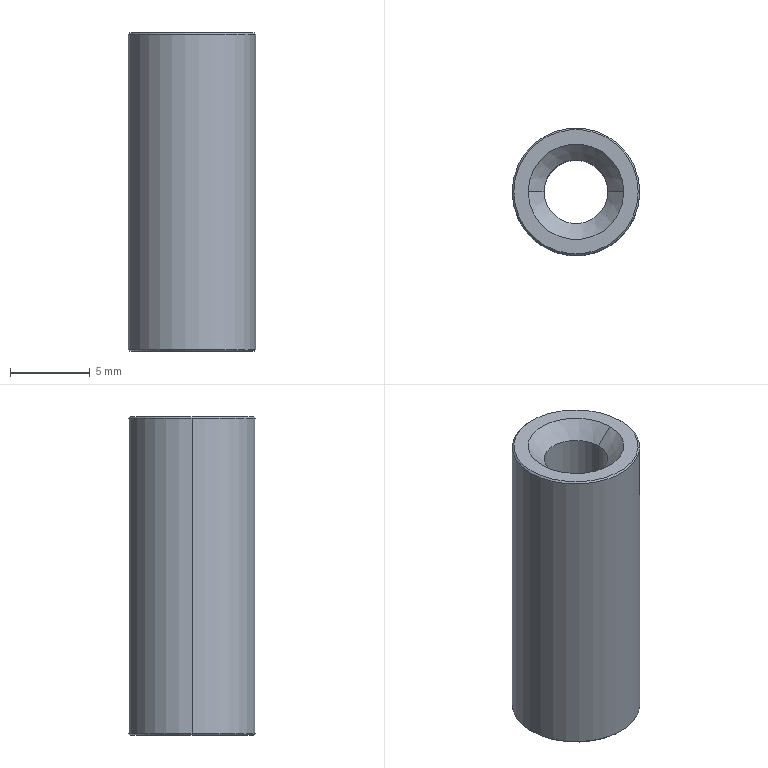Part | NX | features BREP 1 | 1 solid | 14 faces | box 8 x 8 x 20 mm | volume 739.072 mm3 | cone 8 | cylinder 4 | plane 2 | commonest cylinder face diameters 4 x2 8 x2
STEP:
#1=CARTESIAN_POINT('',(2.,0.,1.));
#2=VERTEX_POINT('',#1);
#3=CARTESIAN_POINT('',(-2.,0.,1.));
#4=VERTEX_POINT('',#3);
#5=CARTESIAN_POINT('',(0.,0.,1.));
#6=DIRECTION('',(0.,0.,-1.));
#7=DIRECTION('',(1.,0.,0.));
#8=AXIS2_PLACEMENT_3D('',#5,#6,#7);
#9=CIRCLE('',#8,2.);
#10=EDGE_CURVE('',#2,#4,#9,.T.);
#11=ORIENTED_EDGE('',*,*,#10,.F.);
#12=CARTESIAN_POINT('',(3.,0.,0.));
#13=VERTEX_POINT('',#12);
#14=CARTESIAN_POINT('',(3.,0.,0.));
#15=DIRECTION('',(0.7071,0.,-0.7071));
#16=VECTOR('',#15,1000.);
#17=LINE('',#14,#16);
#18=EDGE_CURVE('',#2,#13,#17,.T.);
#19=ORIENTED_EDGE('',*,*,#18,.T.);
#20=CARTESIAN_POINT('',(-3.,0.,0.));
#21=VERTEX_POINT('',#20);
#22=CARTESIAN_POINT('',(0.,0.,0.));
#23=DIRECTION('',(0.,0.,1.));
#24=DIRECTION('',(1.,0.,0.));
#25=AXIS2_PLACEMENT_3D('',#22,#23,#24);
#26=CIRCLE('',#25,3.);
#27=EDGE_CURVE('',#21,#13,#26,.T.);
#28=ORIENTED_EDGE('',*,*,#27,.F.);
#29=CARTESIAN_POINT('',(-3.,0.,0.));
#30=DIRECTION('',(-0.7071,0.,-0.7071));
#31=VECTOR('',#30,1000.);
#32=LINE('',#29,#31);
#33=EDGE_CURVE('',#4,#21,#32,.T.);
#34=ORIENTED_EDGE('',*,*,#33,.F.);
#35=EDGE_LOOP('',(#11,#19,#28,#34));
#36=FACE_BOUND('',#35,.T.);
#37=CARTESIAN_POINT('',(0.,0.,0.));
#38=DIRECTION('',(0.,0.,-1.));
#39=DIRECTION('',(-1.,0.,0.));
#40=AXIS2_PLACEMENT_3D('',#37,#38,#39);
#41=CONICAL_SURFACE('',#40,3.,0.7854);
#42=ADVANCED_FACE('',(#36),#41,.F.);
#43=CARTESIAN_POINT('',(-2.,0.,19.));
#44=VERTEX_POINT('',#43);
#45=CARTESIAN_POINT('',(2.,0.,19.));
#46=VERTEX_POINT('',#45);
#47=CARTESIAN_POINT('',(0.,0.,19.));
#48=DIRECTION('',(0.,0.,1.));
#49=DIRECTION('',(1.,0.,0.));
#50=AXIS2_PLACEMENT_3D('',#47,#48,#49);
#51=CIRCLE('',#50,2.);
#52=EDGE_CURVE('',#44,#46,#51,.T.);
#53=ORIENTED_EDGE('',*,*,#52,.F.);
#54=CARTESIAN_POINT('',(-3.,0.,20.));
#55=VERTEX_POINT('',#54);
#56=CARTESIAN_POINT('',(-2.,0.,19.));
#57=DIRECTION('',(-0.7071,0.,0.7071));
#58=VECTOR('',#57,1000.);
#59=LINE('',#56,#58);
#60=EDGE_CURVE('',#55,#44,#59,.F.);
#61=ORIENTED_EDGE('',*,*,#60,.F.);
#62=CARTESIAN_POINT('',(3.,0.,20.));
#63=VERTEX_POINT('',#62);
#64=CARTESIAN_POINT('',(0.,0.,20.));
#65=DIRECTION('',(0.,0.,-1.));
#66=DIRECTION('',(1.,0.,0.));
#67=AXIS2_PLACEMENT_3D('',#64,#65,#66);
#68=CIRCLE('',#67,3.);
#69=EDGE_CURVE('',#63,#55,#68,.T.);
#70=ORIENTED_EDGE('',*,*,#69,.F.);
#71=CARTESIAN_POINT('',(2.,0.,19.));
#72=DIRECTION('',(0.7071,0.,0.7071));
#73=VECTOR('',#72,1000.);
#74=LINE('',#71,#73);
#75=EDGE_CURVE('',#63,#46,#74,.F.);
#76=ORIENTED_EDGE('',*,*,#75,.T.);
#77=EDGE_LOOP('',(#53,#61,#70,#76));
#78=FACE_BOUND('',#77,.T.);
#79=CARTESIAN_POINT('',(0.,0.,19.));
#80=DIRECTION('',(0.,0.,1.));
#81=DIRECTION('',(1.,0.,0.));
#82=AXIS2_PLACEMENT_3D('',#79,#80,#81);
#83=CONICAL_SURFACE('',#82,2.,0.7854);
#84=ADVANCED_FACE('',(#78),#83,.F.);
#85=CARTESIAN_POINT('',(3.9,0.,20.));
#86=VERTEX_POINT('',#85);
#87=CARTESIAN_POINT('',(-3.9,0.,20.));
#88=VERTEX_POINT('',#87);
#89=CARTESIAN_POINT('',(0.,0.,20.));
#90=DIRECTION('',(0.,0.,1.));
#91=DIRECTION('',(1.,0.,0.));
#92=AXIS2_PLACEMENT_3D('',#89,#90,#91);
#93=CIRCLE('',#92,3.9);
#94=EDGE_CURVE('',#86,#88,#93,.T.);
#95=ORIENTED_EDGE('',*,*,#94,.F.);
#96=CARTESIAN_POINT('',(4.,0.,19.9));
#97=VERTEX_POINT('',#96);
#98=CARTESIAN_POINT('',(3.9,0.,20.));
#99=DIRECTION('',(0.7071,0.,-0.7071));
#100=VECTOR('',#99,1000.);
#101=LINE('',#98,#100);
#102=EDGE_CURVE('',#86,#97,#101,.T.);
#103=ORIENTED_EDGE('',*,*,#102,.T.);
#104=CARTESIAN_POINT('',(-4.,0.,19.9));
#105=VERTEX_POINT('',#104);
#106=CARTESIAN_POINT('',(0.,0.,19.9));
#107=DIRECTION('',(0.,0.,-1.));
#108=DIRECTION('',(1.,0.,0.));
#109=AXIS2_PLACEMENT_3D('',#106,#107,#108);
#110=CIRCLE('',#109,4.);
#111=EDGE_CURVE('',#105,#97,#110,.T.);
#112=ORIENTED_EDGE('',*,*,#111,.F.);
#113=CARTESIAN_POINT('',(-3.9,0.,20.));
#114=DIRECTION('',(-0.7071,0.,-0.7071));
#115=VECTOR('',#114,1000.);
#116=LINE('',#113,#115);
#117=EDGE_CURVE('',#88,#105,#116,.T.);
#118=ORIENTED_EDGE('',*,*,#117,.F.);
#119=EDGE_LOOP('',(#95,#103,#112,#118));
#120=FACE_BOUND('',#119,.T.);
#121=CARTESIAN_POINT('',(0.,0.,20.));
#122=DIRECTION('',(0.,0.,-1.));
#123=DIRECTION('',(-1.,0.,0.));
#124=AXIS2_PLACEMENT_3D('',#121,#122,#123);
#125=CONICAL_SURFACE('',#124,3.9,0.7854);
#126=ADVANCED_FACE('',(#120),#125,.T.);
#127=CARTESIAN_POINT('',(-3.9,0.,0.));
#128=VERTEX_POINT('',#127);
#129=CARTESIAN_POINT('',(3.9,0.,0.));
#130=VERTEX_POINT('',#129);
#131=CARTESIAN_POINT('',(0.,0.,0.));
#132=DIRECTION('',(0.,0.,-1.));
#133=DIRECTION('',(1.,0.,0.));
#134=AXIS2_PLACEMENT_3D('',#131,#132,#133);
#135=CIRCLE('',#134,3.9);
#136=EDGE_CURVE('',#128,#130,#135,.T.);
#137=ORIENTED_EDGE('',*,*,#136,.F.);
#138=CARTESIAN_POINT('',(-4.,0.,0.1));
#139=VERTEX_POINT('',#138);
#140=CARTESIAN_POINT('',(-4.,0.,0.1));
#141=DIRECTION('',(-0.7071,0.,0.7071));
#142=VECTOR('',#141,1000.);
#143=LINE('',#140,#142);
#144=EDGE_CURVE('',#139,#128,#143,.F.);
#145=ORIENTED_EDGE('',*,*,#144,.F.);
#146=CARTESIAN_POINT('',(4.,0.,0.1));
#147=VERTEX_POINT('',#146);
#148=CARTESIAN_POINT('',(0.,0.,0.1));
#149=DIRECTION('',(0.,0.,1.));
#150=DIRECTION('',(1.,0.,0.));
#151=AXIS2_PLACEMENT_3D('',#148,#149,#150);
#152=CIRCLE('',#151,4.);
#153=EDGE_CURVE('',#147,#139,#152,.T.);
#154=ORIENTED_EDGE('',*,*,#153,.F.);
#155=CARTESIAN_POINT('',(4.,0.,0.1));
#156=DIRECTION('',(0.7071,0.,0.7071));
#157=VECTOR('',#156,1000.);
#158=LINE('',#155,#157);
#159=EDGE_CURVE('',#147,#130,#158,.F.);
#160=ORIENTED_EDGE('',*,*,#159,.T.);
#161=EDGE_LOOP('',(#137,#145,#154,#160));
#162=FACE_BOUND('',#161,.T.);
#163=CARTESIAN_POINT('',(0.,0.,0.1));
#164=DIRECTION('',(0.,0.,1.));
#165=DIRECTION('',(1.,0.,0.));
#166=AXIS2_PLACEMENT_3D('',#163,#164,#165);
#167=CONICAL_SURFACE('',#166,4.,0.7854);
#168=ADVANCED_FACE('',(#162),#167,.T.);
#169=ORIENTED_EDGE('',*,*,#52,.T.);
#170=CARTESIAN_POINT('',(2.,0.,20.));
#171=DIRECTION('',(0.,0.,-1.));
#172=VECTOR('',#171,1000.);
#173=LINE('',#170,#172);
#174=EDGE_CURVE('',#46,#2,#173,.T.);
#175=ORIENTED_EDGE('',*,*,#174,.T.);
#176=ORIENTED_EDGE('',*,*,#10,.T.);
#177=CARTESIAN_POINT('',(-2.,0.,20.));
#178=DIRECTION('',(0.,0.,-1.));
#179=VECTOR('',#178,1000.);
#180=LINE('',#177,#179);
#181=EDGE_CURVE('',#44,#4,#180,.T.);
#182=ORIENTED_EDGE('',*,*,#181,.F.);
#183=EDGE_LOOP('',(#169,#175,#176,#182));
#184=FACE_BOUND('',#183,.T.);
#185=CARTESIAN_POINT('',(0.,0.,20.));
#186=DIRECTION('',(0.,0.,-1.));
#187=DIRECTION('',(-1.,0.,0.));
#188=AXIS2_PLACEMENT_3D('',#185,#186,#187);
#189=CYLINDRICAL_SURFACE('',#188,2.);
#190=ADVANCED_FACE('',(#184),#189,.F.);
#191=ORIENTED_EDGE('',*,*,#111,.T.);
#192=CARTESIAN_POINT('',(4.,0.,20.));
#193=DIRECTION('',(0.,0.,-1.));
#194=VECTOR('',#193,1000.);
#195=LINE('',#192,#194);
#196=EDGE_CURVE('',#97,#147,#195,.T.);
#197=ORIENTED_EDGE('',*,*,#196,.T.);
#198=ORIENTED_EDGE('',*,*,#153,.T.);
#199=CARTESIAN_POINT('',(-4.,0.,20.));
#200=DIRECTION('',(0.,0.,-1.));
#201=VECTOR('',#200,1000.);
#202=LINE('',#199,#201);
#203=EDGE_CURVE('',#105,#139,#202,.T.);
#204=ORIENTED_EDGE('',*,*,#203,.F.);
#205=EDGE_LOOP('',(#191,#197,#198,#204));
#206=FACE_BOUND('',#205,.T.);
#207=CARTESIAN_POINT('',(0.,0.,20.));
#208=DIRECTION('',(0.,0.,-1.));
#209=DIRECTION('',(-1.,0.,0.));
#210=AXIS2_PLACEMENT_3D('',#207,#208,#209);
#211=CYLINDRICAL_SURFACE('',#210,4.);
#212=ADVANCED_FACE('',(#206),#211,.T.);
#213=CARTESIAN_POINT('',(0.,0.,20.));
#214=DIRECTION('',(0.,0.,1.));
#215=DIRECTION('',(1.,0.,0.));
#216=AXIS2_PLACEMENT_3D('',#213,#214,#215);
#217=CIRCLE('',#216,3.9);
#218=EDGE_CURVE('',#88,#86,#217,.T.);
#219=ORIENTED_EDGE('',*,*,#218,.T.);
#220=ORIENTED_EDGE('',*,*,#94,.T.);
#221=EDGE_LOOP('',(#219,#220));
#222=FACE_BOUND('',#221,.T.);
#223=ORIENTED_EDGE('',*,*,#69,.T.);
#224=CARTESIAN_POINT('',(0.,0.,20.));
#225=DIRECTION('',(0.,0.,-1.));
#226=DIRECTION('',(1.,0.,0.));
#227=AXIS2_PLACEMENT_3D('',#224,#225,#226);
#228=CIRCLE('',#227,3.);
#229=EDGE_CURVE('',#55,#63,#228,.T.);
#230=ORIENTED_EDGE('',*,*,#229,.T.);
#231=EDGE_LOOP('',(#223,#230));
#232=FACE_BOUND('',#231,.T.);
#233=CARTESIAN_POINT('',(0.,0.,20.));
#234=DIRECTION('',(0.,0.,1.));
#235=DIRECTION('',(1.,0.,0.));
#236=AXIS2_PLACEMENT_3D('',#233,#234,#235);
#237=PLANE('',#236);
#238=ADVANCED_FACE('',(#222,#232),#237,.T.);
#239=CARTESIAN_POINT('',(0.,0.,0.));
#240=DIRECTION('',(0.,0.,-1.));
#241=DIRECTION('',(1.,0.,0.));
#242=AXIS2_PLACEMENT_3D('',#239,#240,#241);
#243=CIRCLE('',#242,3.9);
#244=EDGE_CURVE('',#130,#128,#243,.T.);
#245=ORIENTED_EDGE('',*,*,#244,.T.);
#246=ORIENTED_EDGE('',*,*,#136,.T.);
#247=EDGE_LOOP('',(#245,#246));
#248=FACE_BOUND('',#247,.T.);
#249=ORIENTED_EDGE('',*,*,#27,.T.);
#250=CARTESIAN_POINT('',(0.,0.,0.));
#251=DIRECTION('',(0.,0.,1.));
#252=DIRECTION('',(1.,0.,0.));
#253=AXIS2_PLACEMENT_3D('',#250,#251,#252);
#254=CIRCLE('',#253,3.);
#255=EDGE_CURVE('',#13,#21,#254,.T.);
#256=ORIENTED_EDGE('',*,*,#255,.T.);
#257=EDGE_LOOP('',(#249,#256));
#258=FACE_BOUND('',#257,.T.);
#259=CARTESIAN_POINT('',(0.,0.,0.));
#260=DIRECTION('',(0.,0.,1.));
#261=DIRECTION('',(1.,0.,0.));
#262=AXIS2_PLACEMENT_3D('',#259,#260,#261);
#263=PLANE('',#262);
#264=ADVANCED_FACE('',(#248,#258),#263,.F.);
#265=ORIENTED_EDGE('',*,*,#196,.F.);
#266=CARTESIAN_POINT('',(0.,0.,19.9));
#267=DIRECTION('',(0.,0.,-1.));
#268=DIRECTION('',(1.,0.,0.));
#269=AXIS2_PLACEMENT_3D('',#266,#267,#268);
#270=CIRCLE('',#269,4.);
#271=EDGE_CURVE('',#97,#105,#270,.T.);
#272=ORIENTED_EDGE('',*,*,#271,.T.);
#273=ORIENTED_EDGE('',*,*,#203,.T.);
#274=CARTESIAN_POINT('',(0.,0.,0.1));
#275=DIRECTION('',(0.,0.,1.));
#276=DIRECTION('',(1.,0.,0.));
#277=AXIS2_PLACEMENT_3D('',#274,#275,#276);
#278=CIRCLE('',#277,4.);
#279=EDGE_CURVE('',#139,#147,#278,.T.);
#280=ORIENTED_EDGE('',*,*,#279,.T.);
#281=EDGE_LOOP('',(#265,#272,#273,#280));
#282=FACE_BOUND('',#281,.T.);
#283=CARTESIAN_POINT('',(0.,0.,20.));
#284=DIRECTION('',(0.,0.,-1.));
#285=DIRECTION('',(-1.,0.,0.));
#286=AXIS2_PLACEMENT_3D('',#283,#284,#285);
#287=CYLINDRICAL_SURFACE('',#286,4.);
#288=ADVANCED_FACE('',(#282),#287,.T.);
#289=ORIENTED_EDGE('',*,*,#174,.F.);
#290=CARTESIAN_POINT('',(0.,0.,19.));
#291=DIRECTION('',(0.,0.,1.));
#292=DIRECTION('',(1.,0.,0.));
#293=AXIS2_PLACEMENT_3D('',#290,#291,#292);
#294=CIRCLE('',#293,2.);
#295=EDGE_CURVE('',#46,#44,#294,.T.);
#296=ORIENTED_EDGE('',*,*,#295,.T.);
#297=ORIENTED_EDGE('',*,*,#181,.T.);
#298=CARTESIAN_POINT('',(0.,0.,1.));
#299=DIRECTION('',(0.,0.,-1.));
#300=DIRECTION('',(1.,0.,0.));
#301=AXIS2_PLACEMENT_3D('',#298,#299,#300);
#302=CIRCLE('',#301,2.);
#303=EDGE_CURVE('',#4,#2,#302,.T.);
#304=ORIENTED_EDGE('',*,*,#303,.T.);
#305=EDGE_LOOP('',(#289,#296,#297,#304));
#306=FACE_BOUND('',#305,.T.);
#307=CARTESIAN_POINT('',(0.,0.,20.));
#308=DIRECTION('',(0.,0.,-1.));
#309=DIRECTION('',(-1.,0.,0.));
#310=AXIS2_PLACEMENT_3D('',#307,#308,#309);
#311=CYLINDRICAL_SURFACE('',#310,2.);
#312=ADVANCED_FACE('',(#306),#311,.F.);
#313=ORIENTED_EDGE('',*,*,#144,.T.);
#314=ORIENTED_EDGE('',*,*,#244,.F.);
#315=ORIENTED_EDGE('',*,*,#159,.F.);
#316=ORIENTED_EDGE('',*,*,#279,.F.);
#317=EDGE_LOOP('',(#313,#314,#315,#316));
#318=FACE_BOUND('',#317,.T.);
#319=CARTESIAN_POINT('',(0.,0.,0.1));
#320=DIRECTION('',(0.,0.,1.));
#321=DIRECTION('',(1.,0.,0.));
#322=AXIS2_PLACEMENT_3D('',#319,#320,#321);
#323=CONICAL_SURFACE('',#322,4.,0.7854);
#324=ADVANCED_FACE('',(#318),#323,.T.);
#325=ORIENTED_EDGE('',*,*,#102,.F.);
#326=ORIENTED_EDGE('',*,*,#218,.F.);
#327=ORIENTED_EDGE('',*,*,#117,.T.);
#328=ORIENTED_EDGE('',*,*,#271,.F.);
#329=EDGE_LOOP('',(#325,#326,#327,#328));
#330=FACE_BOUND('',#329,.T.);
#331=CARTESIAN_POINT('',(0.,0.,20.));
#332=DIRECTION('',(0.,0.,-1.));
#333=DIRECTION('',(-1.,0.,0.));
#334=AXIS2_PLACEMENT_3D('',#331,#332,#333);
#335=CONICAL_SURFACE('',#334,3.9,0.7854);
#336=ADVANCED_FACE('',(#330),#335,.T.);
#337=ORIENTED_EDGE('',*,*,#60,.T.);
#338=ORIENTED_EDGE('',*,*,#295,.F.);
#339=ORIENTED_EDGE('',*,*,#75,.F.);
#340=ORIENTED_EDGE('',*,*,#229,.F.);
#341=EDGE_LOOP('',(#337,#338,#339,#340));
#342=FACE_BOUND('',#341,.T.);
#343=CARTESIAN_POINT('',(0.,0.,19.));
#344=DIRECTION('',(0.,0.,1.));
#345=DIRECTION('',(1.,0.,0.));
#346=AXIS2_PLACEMENT_3D('',#343,#344,#345);
#347=CONICAL_SURFACE('',#346,2.,0.7854);
#348=ADVANCED_FACE('',(#342),#347,.F.);
#349=ORIENTED_EDGE('',*,*,#18,.F.);
#350=ORIENTED_EDGE('',*,*,#303,.F.);
#351=ORIENTED_EDGE('',*,*,#33,.T.);
#352=ORIENTED_EDGE('',*,*,#255,.F.);
#353=EDGE_LOOP('',(#349,#350,#351,#352));
#354=FACE_BOUND('',#353,.T.);
#355=CARTESIAN_POINT('',(0.,0.,0.));
#356=DIRECTION('',(0.,0.,-1.));
#357=DIRECTION('',(-1.,0.,0.));
#358=AXIS2_PLACEMENT_3D('',#355,#356,#357);
#359=CONICAL_SURFACE('',#358,3.,0.7854);
#360=ADVANCED_FACE('',(#354),#359,.F.);
#361=CLOSED_SHELL('',(#42,#84,#126,#168,#190,#212,#238,#264,#288,#312,#324,#336,#348,#360));
#362=MANIFOLD_SOLID_BREP('',#361);
#363=(LENGTH_UNIT()NAMED_UNIT(*)SI_UNIT(.MILLI.,.METRE.));
#364=UNCERTAINTY_MEASURE_WITH_UNIT(LENGTH_MEASURE(0.00001),#363,'','');
#365=(NAMED_UNIT(*)PLANE_ANGLE_UNIT()SI_UNIT($,.RADIAN.));
#366=(NAMED_UNIT(*)SI_UNIT($,.STERADIAN.)SOLID_ANGLE_UNIT());
#367=(GEOMETRIC_REPRESENTATION_CONTEXT(3)GLOBAL_UNCERTAINTY_ASSIGNED_CONTEXT((#364))GLOBAL_UNIT_ASSIGNED_CONTEXT((#363,#365,#366))REPRESENTATION_CONTEXT('',''));
#368=ADVANCED_BREP_SHAPE_REPRESENTATION('',(#362),#367);